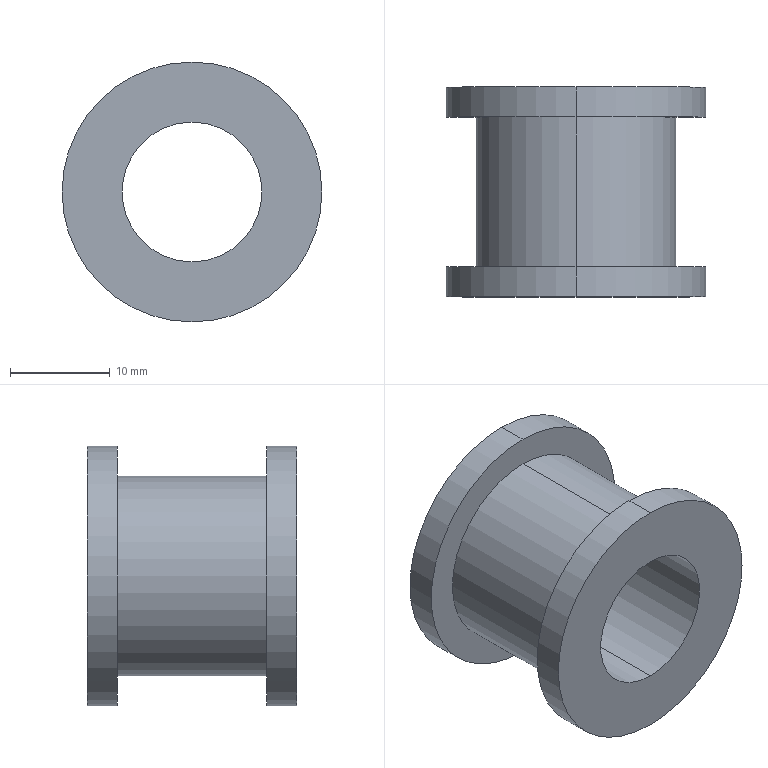Part | SolidWorks | features BaseBody 1 | 1 solid | 12 faces | box 26 x 21 x 26 mm | volume 4665 mm3 | cylinder 8 | plane 4 | commonest cylinder face diameters 26 x4 14 x2 20 x2
STEP:
#1=CARTESIAN_POINT('',(-43.753,648.757,-309.268));
#2=VERTEX_POINT('',#1);
#3=CARTESIAN_POINT('',(-43.753,648.757,-289.268));
#4=VERTEX_POINT('',#3);
#5=CARTESIAN_POINT('',(-43.753,648.757,-299.268));
#6=DIRECTION('',(0.,-1.,0.));
#7=DIRECTION('',(0.,0.,-1.));
#8=AXIS2_PLACEMENT_3D('',#5,#6,#7);
#9=CIRCLE('',#8,10.);
#10=EDGE_CURVE('',#2,#4,#9,.T.);
#11=ORIENTED_EDGE('',*,*,#10,.T.);
#12=CARTESIAN_POINT('',(-43.753,633.757,-289.268));
#13=VERTEX_POINT('',#12);
#14=CARTESIAN_POINT('',(-43.753,656.757,-289.268));
#15=DIRECTION('',(0.,-1.,0.));
#16=VECTOR('',#15,1000.);
#17=LINE('',#14,#16);
#18=EDGE_CURVE('',#4,#13,#17,.T.);
#19=ORIENTED_EDGE('',*,*,#18,.T.);
#20=CARTESIAN_POINT('',(-43.753,633.757,-309.268));
#21=VERTEX_POINT('',#20);
#22=CARTESIAN_POINT('',(-43.753,633.757,-299.268));
#23=DIRECTION('',(0.,1.,0.));
#24=DIRECTION('',(0.,0.,-1.));
#25=AXIS2_PLACEMENT_3D('',#22,#23,#24);
#26=CIRCLE('',#25,10.);
#27=EDGE_CURVE('',#13,#21,#26,.T.);
#28=ORIENTED_EDGE('',*,*,#27,.T.);
#29=CARTESIAN_POINT('',(-43.753,656.757,-309.268));
#30=DIRECTION('',(0.,-1.,0.));
#31=VECTOR('',#30,1000.);
#32=LINE('',#29,#31);
#33=EDGE_CURVE('',#2,#21,#32,.T.);
#34=ORIENTED_EDGE('',*,*,#33,.F.);
#35=EDGE_LOOP('',(#11,#19,#28,#34));
#36=FACE_OUTER_BOUND('',#35,.T.);
#37=CARTESIAN_POINT('',(-43.753,656.757,-299.268));
#38=DIRECTION('',(0.,-1.,0.));
#39=DIRECTION('',(0.,0.,-1.));
#40=AXIS2_PLACEMENT_3D('',#37,#38,#39);
#41=CYLINDRICAL_SURFACE('',#40,10.);
#42=ADVANCED_FACE('',(#36),#41,.T.);
#43=CARTESIAN_POINT('',(-43.753,651.757,-312.268));
#44=VERTEX_POINT('',#43);
#45=CARTESIAN_POINT('',(-43.753,651.757,-286.268));
#46=VERTEX_POINT('',#45);
#47=CARTESIAN_POINT('',(-43.753,651.757,-299.268));
#48=DIRECTION('',(0.,-1.,0.));
#49=DIRECTION('',(0.,0.,-1.));
#50=AXIS2_PLACEMENT_3D('',#47,#48,#49);
#51=CIRCLE('',#50,13.);
#52=EDGE_CURVE('',#44,#46,#51,.T.);
#53=ORIENTED_EDGE('',*,*,#52,.T.);
#54=CARTESIAN_POINT('',(-43.753,648.757,-286.268));
#55=VERTEX_POINT('',#54);
#56=CARTESIAN_POINT('',(-43.753,651.757,-286.268));
#57=DIRECTION('',(0.,-1.,0.));
#58=VECTOR('',#57,1000.);
#59=LINE('',#56,#58);
#60=EDGE_CURVE('',#46,#55,#59,.T.);
#61=ORIENTED_EDGE('',*,*,#60,.T.);
#62=CARTESIAN_POINT('',(-43.753,648.757,-312.268));
#63=VERTEX_POINT('',#62);
#64=CARTESIAN_POINT('',(-43.753,648.757,-299.268));
#65=DIRECTION('',(0.,1.,0.));
#66=DIRECTION('',(0.,0.,-1.));
#67=AXIS2_PLACEMENT_3D('',#64,#65,#66);
#68=CIRCLE('',#67,13.);
#69=EDGE_CURVE('',#55,#63,#68,.T.);
#70=ORIENTED_EDGE('',*,*,#69,.T.);
#71=CARTESIAN_POINT('',(-43.753,651.757,-312.268));
#72=DIRECTION('',(0.,-1.,0.));
#73=VECTOR('',#72,1000.);
#74=LINE('',#71,#73);
#75=EDGE_CURVE('',#44,#63,#74,.T.);
#76=ORIENTED_EDGE('',*,*,#75,.F.);
#77=EDGE_LOOP('',(#53,#61,#70,#76));
#78=FACE_OUTER_BOUND('',#77,.T.);
#79=CARTESIAN_POINT('',(-43.753,651.757,-299.268));
#80=DIRECTION('',(0.,-1.,0.));
#81=DIRECTION('',(0.,0.,-1.));
#82=AXIS2_PLACEMENT_3D('',#79,#80,#81);
#83=CYLINDRICAL_SURFACE('',#82,13.);
#84=ADVANCED_FACE('',(#78),#83,.T.);
#85=CARTESIAN_POINT('',(-43.753,633.757,-286.268));
#86=VERTEX_POINT('',#85);
#87=CARTESIAN_POINT('',(-43.753,633.757,-312.268));
#88=VERTEX_POINT('',#87);
#89=CARTESIAN_POINT('',(-43.753,633.757,-299.268));
#90=DIRECTION('',(0.,1.,0.));
#91=DIRECTION('',(0.,0.,-1.));
#92=AXIS2_PLACEMENT_3D('',#89,#90,#91);
#93=CIRCLE('',#92,13.);
#94=EDGE_CURVE('',#86,#88,#93,.T.);
#95=ORIENTED_EDGE('',*,*,#94,.F.);
#96=CARTESIAN_POINT('',(-43.753,630.757,-286.268));
#97=VERTEX_POINT('',#96);
#98=CARTESIAN_POINT('',(-43.753,656.757,-286.268));
#99=DIRECTION('',(0.,-1.,0.));
#100=VECTOR('',#99,1000.);
#101=LINE('',#98,#100);
#102=EDGE_CURVE('',#86,#97,#101,.T.);
#103=ORIENTED_EDGE('',*,*,#102,.T.);
#104=CARTESIAN_POINT('',(-43.753,630.757,-312.268));
#105=VERTEX_POINT('',#104);
#106=CARTESIAN_POINT('',(-43.753,630.757,-299.268));
#107=DIRECTION('',(0.,1.,0.));
#108=DIRECTION('',(0.,0.,-1.));
#109=AXIS2_PLACEMENT_3D('',#106,#107,#108);
#110=CIRCLE('',#109,13.);
#111=EDGE_CURVE('',#97,#105,#110,.T.);
#112=ORIENTED_EDGE('',*,*,#111,.T.);
#113=CARTESIAN_POINT('',(-43.753,656.757,-312.268));
#114=DIRECTION('',(0.,-1.,0.));
#115=VECTOR('',#114,1000.);
#116=LINE('',#113,#115);
#117=EDGE_CURVE('',#88,#105,#116,.T.);
#118=ORIENTED_EDGE('',*,*,#117,.F.);
#119=EDGE_LOOP('',(#95,#103,#112,#118));
#120=FACE_OUTER_BOUND('',#119,.T.);
#121=CARTESIAN_POINT('',(-43.753,656.757,-299.268));
#122=DIRECTION('',(0.,-1.,0.));
#123=DIRECTION('',(0.,0.,-1.));
#124=AXIS2_PLACEMENT_3D('',#121,#122,#123);
#125=CYLINDRICAL_SURFACE('',#124,13.);
#126=ADVANCED_FACE('',(#120),#125,.T.);
#127=CARTESIAN_POINT('',(-43.753,651.757,-292.268));
#128=VERTEX_POINT('',#127);
#129=CARTESIAN_POINT('',(-43.753,651.757,-306.268));
#130=VERTEX_POINT('',#129);
#131=CARTESIAN_POINT('',(-43.753,651.757,-299.268));
#132=DIRECTION('',(0.,-1.,0.));
#133=DIRECTION('',(0.,0.,-1.));
#134=AXIS2_PLACEMENT_3D('',#131,#132,#133);
#135=CIRCLE('',#134,7.);
#136=EDGE_CURVE('',#128,#130,#135,.T.);
#137=ORIENTED_EDGE('',*,*,#136,.F.);
#138=CARTESIAN_POINT('',(-43.753,630.757,-292.268));
#139=VERTEX_POINT('',#138);
#140=CARTESIAN_POINT('',(-43.753,643.757,-292.268));
#141=DIRECTION('',(0.,-1.,0.));
#142=VECTOR('',#141,1000.);
#143=LINE('',#140,#142);
#144=EDGE_CURVE('',#128,#139,#143,.T.);
#145=ORIENTED_EDGE('',*,*,#144,.T.);
#146=CARTESIAN_POINT('',(-43.753,630.757,-306.268));
#147=VERTEX_POINT('',#146);
#148=CARTESIAN_POINT('',(-43.753,630.757,-299.268));
#149=DIRECTION('',(0.,1.,0.));
#150=DIRECTION('',(0.,0.,-1.));
#151=AXIS2_PLACEMENT_3D('',#148,#149,#150);
#152=CIRCLE('',#151,7.);
#153=EDGE_CURVE('',#147,#139,#152,.T.);
#154=ORIENTED_EDGE('',*,*,#153,.F.);
#155=CARTESIAN_POINT('',(-43.753,643.757,-306.268));
#156=DIRECTION('',(0.,-1.,0.));
#157=VECTOR('',#156,1000.);
#158=LINE('',#155,#157);
#159=EDGE_CURVE('',#130,#147,#158,.T.);
#160=ORIENTED_EDGE('',*,*,#159,.F.);
#161=EDGE_LOOP('',(#137,#145,#154,#160));
#162=FACE_OUTER_BOUND('',#161,.T.);
#163=CARTESIAN_POINT('',(-43.753,643.757,-299.268));
#164=DIRECTION('',(0.,-1.,0.));
#165=DIRECTION('',(0.,0.,-1.));
#166=AXIS2_PLACEMENT_3D('',#163,#164,#165);
#167=CYLINDRICAL_SURFACE('',#166,7.);
#168=ADVANCED_FACE('',(#162),#167,.F.);
#169=ORIENTED_EDGE('',*,*,#18,.F.);
#170=CARTESIAN_POINT('',(-43.753,648.757,-299.268));
#171=DIRECTION('',(0.,-1.,0.));
#172=DIRECTION('',(0.,0.,-1.));
#173=AXIS2_PLACEMENT_3D('',#170,#171,#172);
#174=CIRCLE('',#173,10.);
#175=EDGE_CURVE('',#4,#2,#174,.T.);
#176=ORIENTED_EDGE('',*,*,#175,.T.);
#177=ORIENTED_EDGE('',*,*,#33,.T.);
#178=CARTESIAN_POINT('',(-43.753,633.757,-299.268));
#179=DIRECTION('',(0.,1.,0.));
#180=DIRECTION('',(0.,0.,-1.));
#181=AXIS2_PLACEMENT_3D('',#178,#179,#180);
#182=CIRCLE('',#181,10.);
#183=EDGE_CURVE('',#21,#13,#182,.T.);
#184=ORIENTED_EDGE('',*,*,#183,.T.);
#185=EDGE_LOOP('',(#169,#176,#177,#184));
#186=FACE_OUTER_BOUND('',#185,.T.);
#187=CARTESIAN_POINT('',(-43.753,656.757,-299.268));
#188=DIRECTION('',(0.,-1.,0.));
#189=DIRECTION('',(0.,0.,-1.));
#190=AXIS2_PLACEMENT_3D('',#187,#188,#189);
#191=CYLINDRICAL_SURFACE('',#190,10.);
#192=ADVANCED_FACE('',(#186),#191,.T.);
#193=ORIENTED_EDGE('',*,*,#10,.F.);
#194=ORIENTED_EDGE('',*,*,#175,.F.);
#195=EDGE_LOOP('',(#193,#194));
#196=FACE_BOUND('',#195,.T.);
#197=CARTESIAN_POINT('',(-43.753,648.757,-299.268));
#198=DIRECTION('',(0.,1.,0.));
#199=DIRECTION('',(0.,0.,-1.));
#200=AXIS2_PLACEMENT_3D('',#197,#198,#199);
#201=CIRCLE('',#200,13.);
#202=EDGE_CURVE('',#63,#55,#201,.T.);
#203=ORIENTED_EDGE('',*,*,#202,.F.);
#204=ORIENTED_EDGE('',*,*,#69,.F.);
#205=EDGE_LOOP('',(#203,#204));
#206=FACE_OUTER_BOUND('',#205,.T.);
#207=CARTESIAN_POINT('',(-43.753,648.757,-299.268));
#208=DIRECTION('',(0.,1.,0.));
#209=DIRECTION('',(0.,0.,1.));
#210=AXIS2_PLACEMENT_3D('',#207,#208,#209);
#211=PLANE('',#210);
#212=ADVANCED_FACE('',(#196,#206),#211,.F.);
#213=ORIENTED_EDGE('',*,*,#183,.F.);
#214=ORIENTED_EDGE('',*,*,#27,.F.);
#215=EDGE_LOOP('',(#213,#214));
#216=FACE_BOUND('',#215,.T.);
#217=CARTESIAN_POINT('',(-43.753,633.757,-299.268));
#218=DIRECTION('',(0.,1.,0.));
#219=DIRECTION('',(0.,0.,-1.));
#220=AXIS2_PLACEMENT_3D('',#217,#218,#219);
#221=CIRCLE('',#220,13.);
#222=EDGE_CURVE('',#88,#86,#221,.T.);
#223=ORIENTED_EDGE('',*,*,#222,.T.);
#224=ORIENTED_EDGE('',*,*,#94,.T.);
#225=EDGE_LOOP('',(#223,#224));
#226=FACE_OUTER_BOUND('',#225,.T.);
#227=CARTESIAN_POINT('',(-43.753,633.757,-299.268));
#228=DIRECTION('',(0.,1.,0.));
#229=DIRECTION('',(0.,0.,1.));
#230=AXIS2_PLACEMENT_3D('',#227,#228,#229);
#231=PLANE('',#230);
#232=ADVANCED_FACE('',(#216,#226),#231,.T.);
#233=ORIENTED_EDGE('',*,*,#60,.F.);
#234=CARTESIAN_POINT('',(-43.753,651.757,-299.268));
#235=DIRECTION('',(0.,-1.,0.));
#236=DIRECTION('',(0.,0.,-1.));
#237=AXIS2_PLACEMENT_3D('',#234,#235,#236);
#238=CIRCLE('',#237,13.);
#239=EDGE_CURVE('',#46,#44,#238,.T.);
#240=ORIENTED_EDGE('',*,*,#239,.T.);
#241=ORIENTED_EDGE('',*,*,#75,.T.);
#242=ORIENTED_EDGE('',*,*,#202,.T.);
#243=EDGE_LOOP('',(#233,#240,#241,#242));
#244=FACE_OUTER_BOUND('',#243,.T.);
#245=CARTESIAN_POINT('',(-43.753,651.757,-299.268));
#246=DIRECTION('',(0.,-1.,0.));
#247=DIRECTION('',(0.,0.,-1.));
#248=AXIS2_PLACEMENT_3D('',#245,#246,#247);
#249=CYLINDRICAL_SURFACE('',#248,13.);
#250=ADVANCED_FACE('',(#244),#249,.T.);
#251=ORIENTED_EDGE('',*,*,#102,.F.);
#252=ORIENTED_EDGE('',*,*,#222,.F.);
#253=ORIENTED_EDGE('',*,*,#117,.T.);
#254=CARTESIAN_POINT('',(-43.753,630.757,-299.268));
#255=DIRECTION('',(0.,1.,0.));
#256=DIRECTION('',(0.,0.,-1.));
#257=AXIS2_PLACEMENT_3D('',#254,#255,#256);
#258=CIRCLE('',#257,13.);
#259=EDGE_CURVE('',#105,#97,#258,.T.);
#260=ORIENTED_EDGE('',*,*,#259,.T.);
#261=EDGE_LOOP('',(#251,#252,#253,#260));
#262=FACE_OUTER_BOUND('',#261,.T.);
#263=CARTESIAN_POINT('',(-43.753,656.757,-299.268));
#264=DIRECTION('',(0.,-1.,0.));
#265=DIRECTION('',(0.,0.,-1.));
#266=AXIS2_PLACEMENT_3D('',#263,#264,#265);
#267=CYLINDRICAL_SURFACE('',#266,13.);
#268=ADVANCED_FACE('',(#262),#267,.T.);
#269=CARTESIAN_POINT('',(-43.753,651.757,-299.268));
#270=DIRECTION('',(0.,-1.,0.));
#271=DIRECTION('',(0.,0.,-1.));
#272=AXIS2_PLACEMENT_3D('',#269,#270,#271);
#273=CIRCLE('',#272,7.);
#274=EDGE_CURVE('',#130,#128,#273,.T.);
#275=ORIENTED_EDGE('',*,*,#274,.T.);
#276=ORIENTED_EDGE('',*,*,#136,.T.);
#277=EDGE_LOOP('',(#275,#276));
#278=FACE_BOUND('',#277,.T.);
#279=ORIENTED_EDGE('',*,*,#52,.F.);
#280=ORIENTED_EDGE('',*,*,#239,.F.);
#281=EDGE_LOOP('',(#279,#280));
#282=FACE_OUTER_BOUND('',#281,.T.);
#283=CARTESIAN_POINT('',(-43.753,651.757,-299.268));
#284=DIRECTION('',(0.,1.,0.));
#285=DIRECTION('',(0.,0.,1.));
#286=AXIS2_PLACEMENT_3D('',#283,#284,#285);
#287=PLANE('',#286);
#288=ADVANCED_FACE('',(#278,#282),#287,.T.);
#289=ORIENTED_EDGE('',*,*,#153,.T.);
#290=CARTESIAN_POINT('',(-43.753,630.757,-299.268));
#291=DIRECTION('',(0.,1.,0.));
#292=DIRECTION('',(0.,0.,-1.));
#293=AXIS2_PLACEMENT_3D('',#290,#291,#292);
#294=CIRCLE('',#293,7.);
#295=EDGE_CURVE('',#139,#147,#294,.T.);
#296=ORIENTED_EDGE('',*,*,#295,.T.);
#297=EDGE_LOOP('',(#289,#296));
#298=FACE_BOUND('',#297,.T.);
#299=ORIENTED_EDGE('',*,*,#259,.F.);
#300=ORIENTED_EDGE('',*,*,#111,.F.);
#301=EDGE_LOOP('',(#299,#300));
#302=FACE_OUTER_BOUND('',#301,.T.);
#303=CARTESIAN_POINT('',(-43.753,630.757,-299.268));
#304=DIRECTION('',(0.,-1.,0.));
#305=DIRECTION('',(0.,0.,-1.));
#306=AXIS2_PLACEMENT_3D('',#303,#304,#305);
#307=PLANE('',#306);
#308=ADVANCED_FACE('',(#298,#302),#307,.T.);
#309=ORIENTED_EDGE('',*,*,#144,.F.);
#310=ORIENTED_EDGE('',*,*,#274,.F.);
#311=ORIENTED_EDGE('',*,*,#159,.T.);
#312=ORIENTED_EDGE('',*,*,#295,.F.);
#313=EDGE_LOOP('',(#309,#310,#311,#312));
#314=FACE_OUTER_BOUND('',#313,.T.);
#315=CARTESIAN_POINT('',(-43.753,643.757,-299.268));
#316=DIRECTION('',(0.,-1.,0.));
#317=DIRECTION('',(0.,0.,-1.));
#318=AXIS2_PLACEMENT_3D('',#315,#316,#317);
#319=CYLINDRICAL_SURFACE('',#318,7.);
#320=ADVANCED_FACE('',(#314),#319,.F.);
#321=CLOSED_SHELL('',(#42,#84,#126,#168,#192,#212,#232,#250,#268,#288,#308,#320));
#322=MANIFOLD_SOLID_BREP('',#321);
#323=CARTESIAN_POINT('',(0.,0.,0.));
#324=DIRECTION('',(0.,0.,1.));
#325=DIRECTION('',(1.,0.,0.));
#326=AXIS2_PLACEMENT_3D('',#323,#324,#325);
#327=(LENGTH_UNIT()NAMED_UNIT(*)SI_UNIT(.MILLI.,.METRE.));
#328=UNCERTAINTY_MEASURE_WITH_UNIT(LENGTH_MEASURE(0.00001),#327,'','');
#329=(NAMED_UNIT(*)PLANE_ANGLE_UNIT()SI_UNIT($,.RADIAN.));
#330=(NAMED_UNIT(*)SI_UNIT($,.STERADIAN.)SOLID_ANGLE_UNIT());
#331=(GEOMETRIC_REPRESENTATION_CONTEXT(3)GLOBAL_UNCERTAINTY_ASSIGNED_CONTEXT((#328))GLOBAL_UNIT_ASSIGNED_CONTEXT((#327,#329,#330))REPRESENTATION_CONTEXT('',''));
#332=ADVANCED_BREP_SHAPE_REPRESENTATION('',(#322,#326),#331);